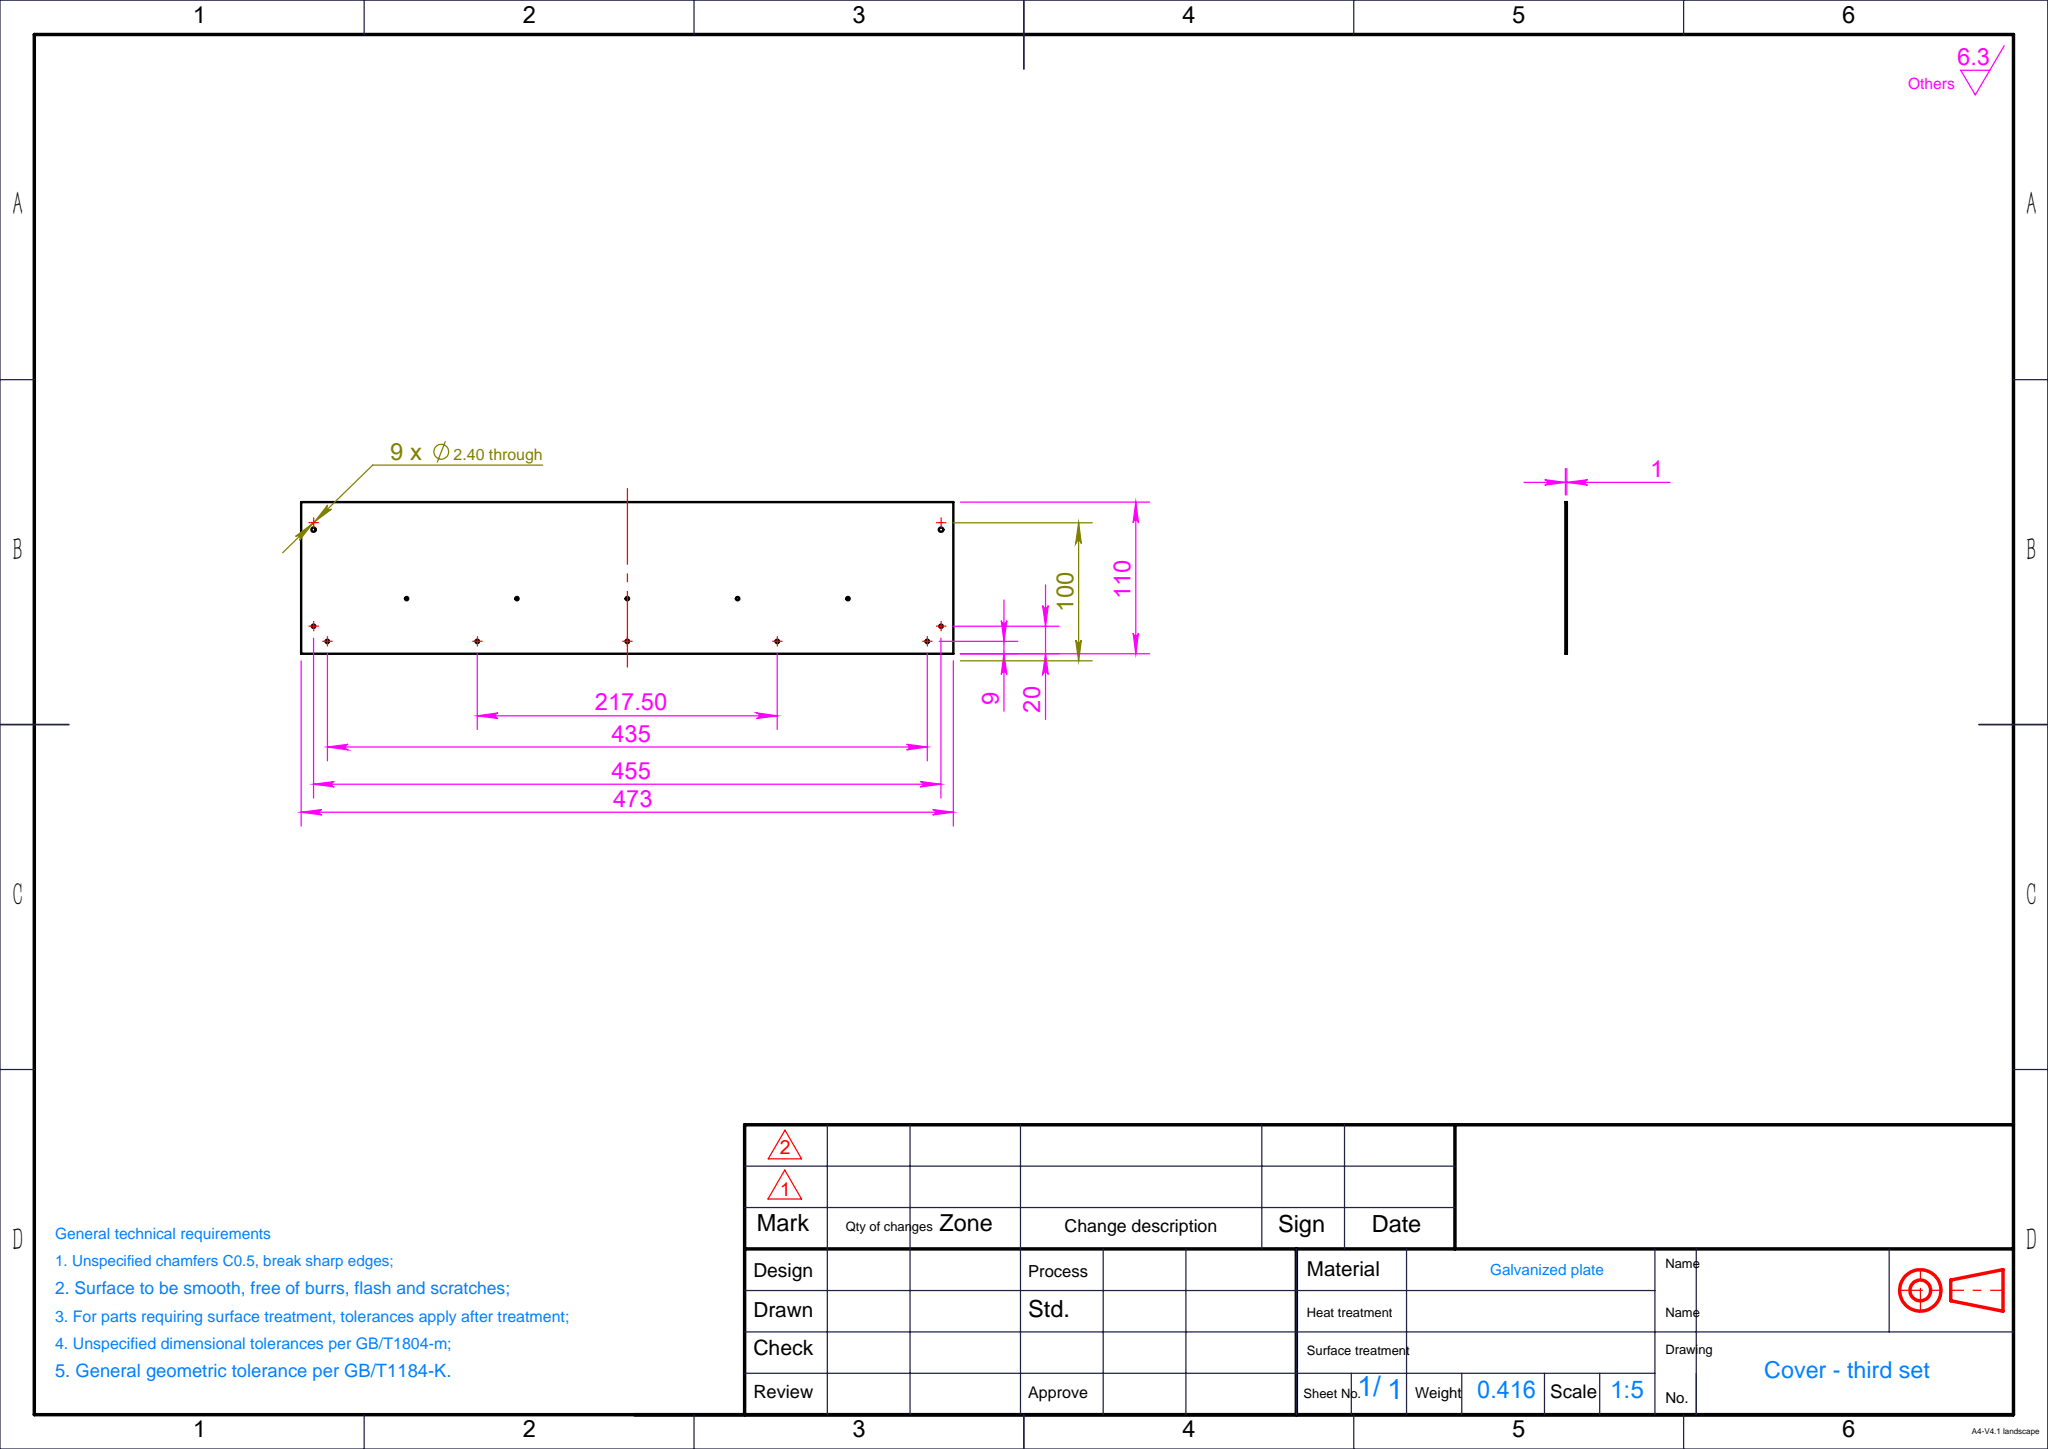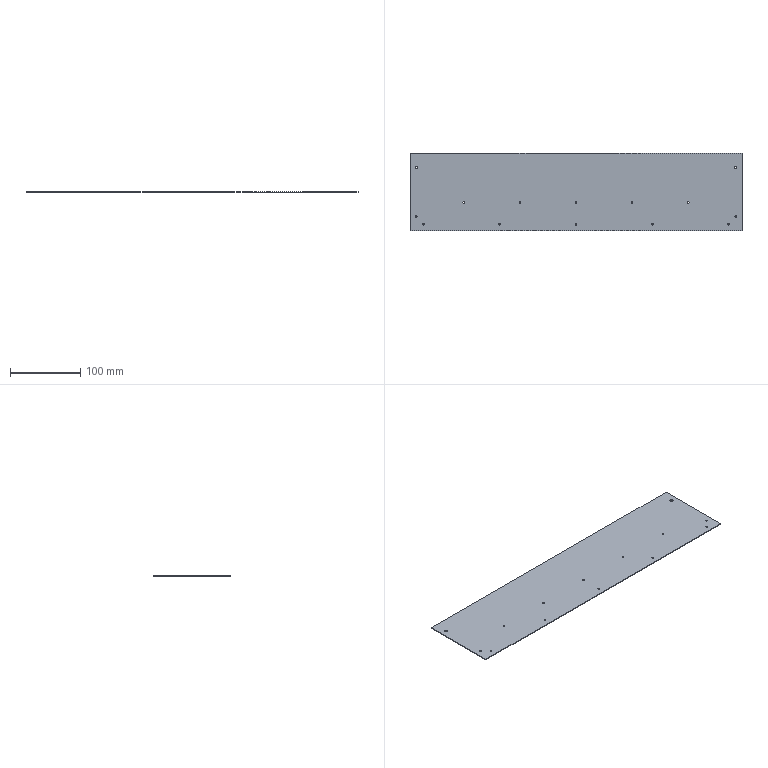Part | SolidWorks | features 3DProfileFeature 1, Chamfer 1, FlatPattern 1, HoleWzd 1, ICE 1, SMBaseFlange 1, SheetMetal 1, SketchPattern 1 | 1 solid | 38 faces | box 473 x 110 x 1 mm | volume 51954 mm3 | cylinder 28 | plane 6 | cone 4 | commonest cylinder face diameters 2.4 x24 3.2 x4